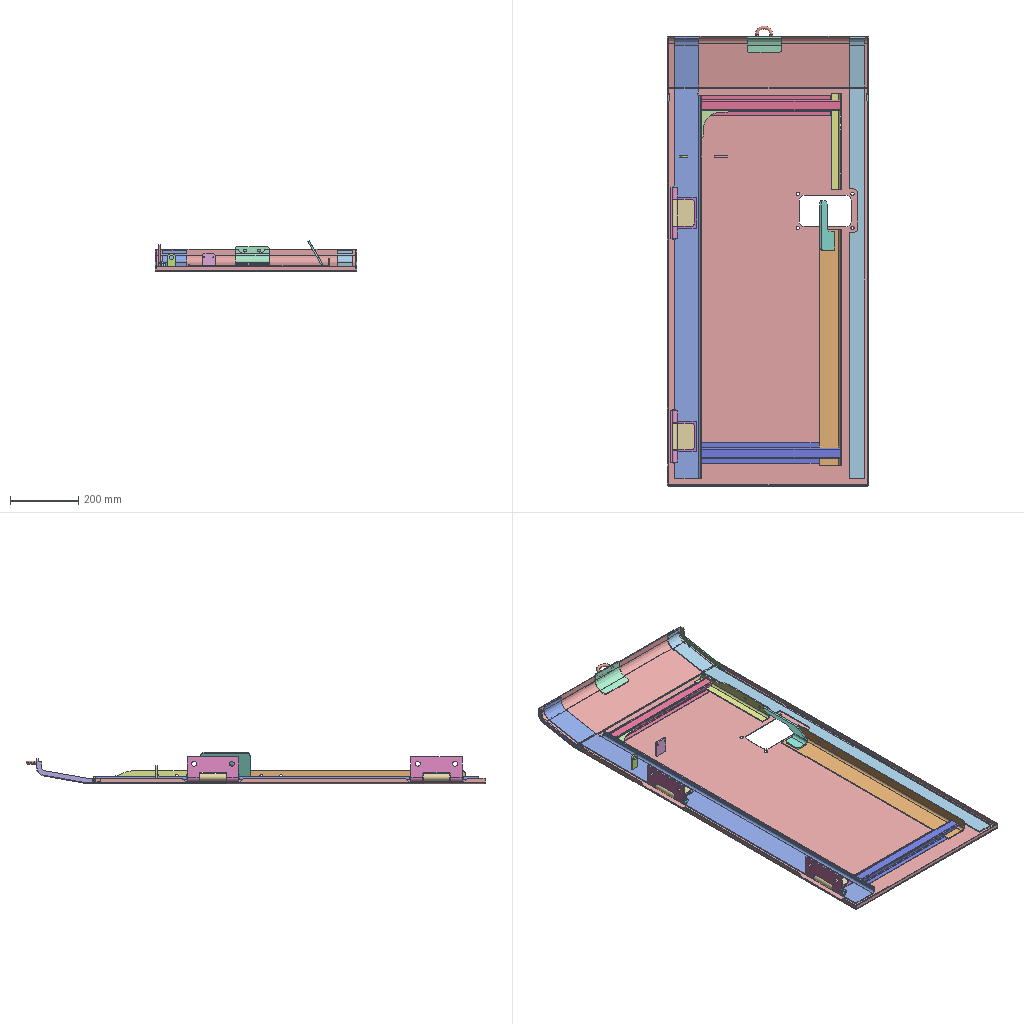Assembly | SolidWorks | 20 different items | 25 placed | box 591 x 1348 x 92 mm
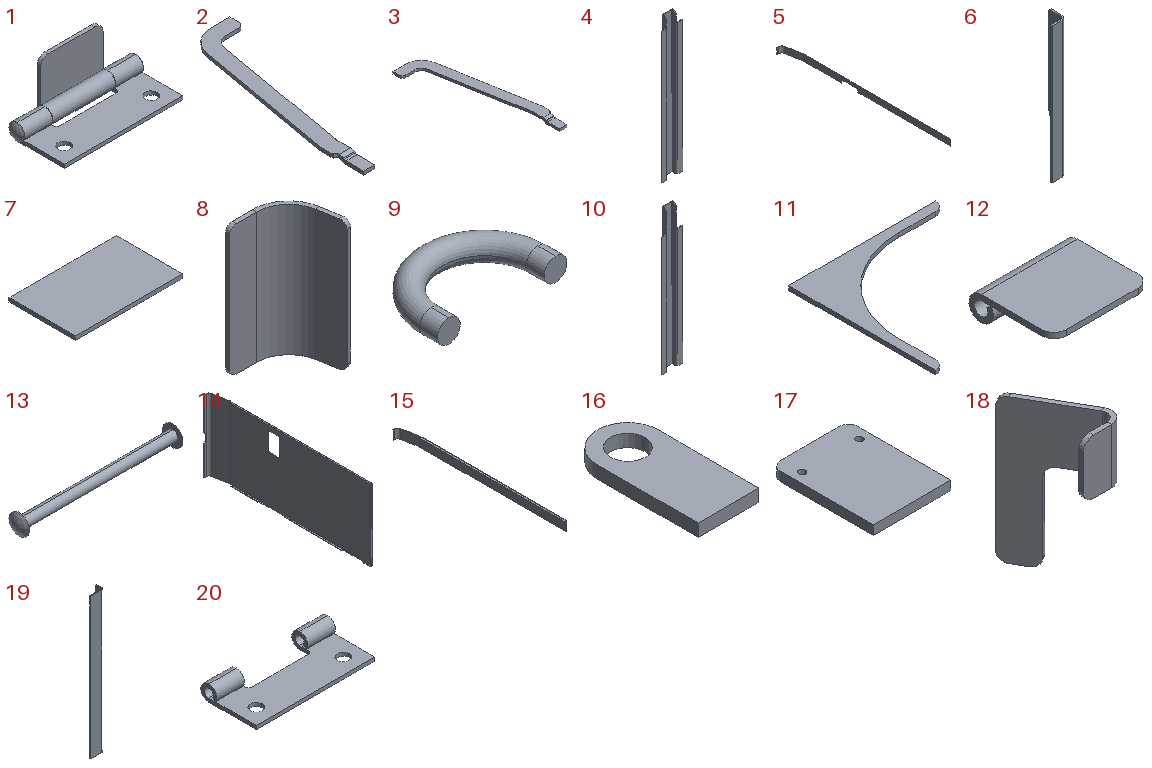Parts list (item | name | quantity | parent item | size | volume | features):
1 | (subassembly) | x2 | - | 157 x 70 x 70 mm | 95055 mm3 | -
2 | - | x1 | - | 63.4 x 186.4 x 5.5 mm | 8701 mm3 | features Fillet 4, FlatPattern 1, ICE 1, SMBaseFlange 1, SheetMetal 1
3 | - | x1 | - | 63.4 x 186.4 x 5.5 mm | 8701 mm3 | features Fillet 4, FlatPattern 1, ICE 1, SMBaseFlange 1, SheetMetal 1
4 | - | x1 | - | 60 x 15 x 406 mm | 52147 mm3 | features ICE 2, Chamfer 1, Fillet 1, FlatPattern 1, SMBaseFlange 1, SheetMetal 1
5 | - | x1 | - | 60.1 x 1293 x 45 mm | 180831 mm3 | features FlatPattern 1, ICE 1, SMBaseFlange 1, SheetMetal 1
6 | - | x1 | - | 30 x 35 x 283 mm | 48637 mm3 | features Fillet 2, FlatPattern 1, ICE 1, SMBaseFlange 1, SheetMetal 1
7 | - | x2 | - | 89 x 55 x 3.2 mm | 15664 mm3 | features FlatPattern 1, SMBaseFlange 1, SheetMetal 1
8 | - | x1 | - | 51.9 x 44.589 x 100 mm | 25102 mm3 | features Fillet 1, FlatPattern 1, SMBaseFlange 1, SheetMetal 1
9 | - | x1 | - | 51 x 32.5 x 9 mm | 5088 mm3 | features Sweep 1
10 | - | x1 | - | 60 x 15 x 406 mm | 50219 mm3 | features ICE 2, Chamfer 1, Fillet 1, FlatPattern 1, SMBaseFlange 1, SheetMetal 1
11 | - | x1 | - | 80 x 80 x 2.3 mm | 2992 mm3 | features Fillet 1, FlatPattern 1, SMBaseFlange 1, SheetMetal 1
12 | - | x2 | in 1 | 79 x 70 x 20 mm | 35683 mm3 | features Fillet 1, FlatPattern 1, SMBaseFlange 1, SheetMetal 1
13 | - | x2 | in 1 | 157 x 20 x 20 mm | 12925 mm3 | features Revolution 1
14 | - | x1 | - | 65.7 x 1318 x 591 mm | 1870359 mm3 | features ICE 4, Chamfer 1, EdgeFlange 1, Fillet 1, FlatPattern 1, SMBaseFlange 1, SheetMetal 1
15 | - | x1 | - | 60.1 x 1293 x 79 mm | 376387 mm3 | features Fillet 2, EdgeFlange 1, FlatPattern 1, ICE 1, SMBaseFlange 1, SheetMetal 1
16 | - | x1 | - | 22 x 47.5 x 4.5 mm | 3917 mm3 | features FlatPattern 1, SMBaseFlange 1, SheetMetal 1
17 | - | x1 | - | 38 x 50 x 4.5 mm | 8425 mm3 | features FlatPattern 1, HoleWzd 1, SMBaseFlange 1, SheetMetal 1
18 | - | x1 | - | 44.746 x 86.603 x 145 mm | 45510 mm3 | features Fillet 1, FlatPattern 1, ICE 1, SMBaseFlange 1, SheetMetal 1
19 | - | x1 | - | 65 x 35 x 690 mm | 206237 mm3 | features Fillet 1, FlatPattern 1, ICE 1, SMBaseFlange 1, SheetMetal 1
20 | - | x2 | in 1 | 150 x 70 x 20 mm | 46447 mm3 | features FlatPattern 1, ICE 1, SMBaseFlange 1, SheetMetal 1
Mates (type | each side: item.copy, entity, surface, feature):
In the top assembly
Coincident | 14.1 face plane Base-Flange1 | 15.1 face plane Base-Flange1 | 2 times
DistanceDim | 15.1 face plane Base-Flange1 | 14.1 face plane Edge-Flange1
Coincident | 15.1 face plane Base-Flange1 | 16.1 face plane Base-Flange1
DistanceDim | 16.1 face plane Base-Flange1 | 14.1 face plane Edge-Flange1
DistanceDim | 16.1 face cylinder Base-Flange1 | 14.1 face plane Edge-Flange1
Coincident | 14.1 face plane Base-Flange1 | 17.1 face plane Base-Flange1
Coincident | 16.1 face plane Base-Flange1 | 17.1 face plane Base-Flange1
DistanceDim | 16.1 face cylinder Base-Flange1 | 17.1 face cylinder M4 Tapped Hole1
DistanceDim | 14.1 face plane Base-Flange1 | 18.1 face plane Base-Flange1
DistanceDim | 14.1 face plane Edge-Flange1 | 18.1 face plane Base-Flange1 | 2 times
Coincident | 14.1 face plane Base-Flange1 | 19.1 face plane Base-Flange1
DistanceDim | 15.1 face plane Edge-Flange1 | 19.1 face plane Base-Flange1
DistanceDim | 14.1 face plane Edge-Flange1 | 19.1 face plane Base-Flange1
Coincident | 14.1 face plane Base-Flange1 | 2.1 face plane Base-Flange1 | 2 times
Coincident | 14.1 face plane Edge-Flange1 | 2.1 face plane Base-Flange1
Coincident | 14.1 face plane Base-Flange1 | 3.1 face plane Base-Flange1 | 2 times
Coincident | 14.1 face plane Edge-Flange1 | 3.1 face plane Base-Flange1
Coincident | 14.1 face plane Base-Flange1 | 4.1 face plane Base-Flange1
Coincident | 15.1 face plane Edge-Flange1 | 4.1 face plane Base-Flange1
DistanceDim | 4.1 face plane Base-Flange1 | 10.1 face plane Base-Flange1
Coincident | 14.1 face plane Base-Flange1 | 5.1 face plane Base-Flange1 | 2 times
DistanceDim | 14.1 face plane Edge-Flange1 | 5.1 face plane Base-Flange1
Coincident | 14.1 face plane Base-Flange1 | 6.1 face plane Base-Flange1
DistanceDim | 6.1 face plane Base-Flange1 | 19.1 face plane Base-Flange1
DistanceDim | 14.1 face plane Edge-Flange1 | 6.1 face plane Base-Flange1
Coincident | 15.1 face plane Base-Flange1 | 7.1 face plane Base-Flange1
DistanceDim | 14.1 face plane Edge-Flange1 | 7.1 face plane Base-Flange1 | 2 times
Coincident | 14.1 face plane Base-Flange1 | 8.1 face plane Base-Flange1
DistanceDim | 8.1 face plane Base-Flange1 | 14.1 face plane Base-Flange1
DistanceDim | 14.1 face plane Edge-Flange1 | 8.1 face plane Base-Flange1
Coincident | 8.1 face plane Base-Flange1 | 9.1 face plane Sweep1
DistanceDim | 8.1 face plane Base-Flange1 | 9.1 face cylinder Sweep1
Coincident | 8.1 plane | 9.1 plane
Coincident | 14.1 face plane Base-Flange1 | 10.1 face plane Base-Flange1
Coincident | 15.1 face plane Edge-Flange1 | 10.1 face plane Base-Flange1
DistanceDim | 14.1 face plane Edge-Flange1 | 10.1 face plane Base-Flange1
Coincident | 15.1 face plane Edge-Flange1 | 11.1 face plane Base-Flange1
Coincident | 4.1 face plane Base-Flange1 | 11.1 face plane Base-Flange1
DistanceDim | 4.1 face plane Base-Flange1 | 11.1 face plane Base-Flange1
Coincident | 7.1 face plane Base-Flange1 | 12.1 face plane Base-Flange1
DistanceDim | 20.1 face cylinder Base-Bend1 | 14.1 face plane Edge-Flange1
DistanceDim | 20.1 face cylinder Cut-Extrude1 | 14.1 face plane Edge-Flange1
In subassembly 1
Concentric | 20.2 face cylinder Base-Bend1 | 13.1 face cylinder Revolve1
Coincident | 20.2 face plane Base-Bend1 | 13.1 face plane Revolve1
Concentric | 13.1 face cylinder Revolve1 | 12.2 face cylinder Base-Bend1
DistanceDim | 12.2 face plane Base-Bend1 | 20.2 face plane Cut-Extrude1